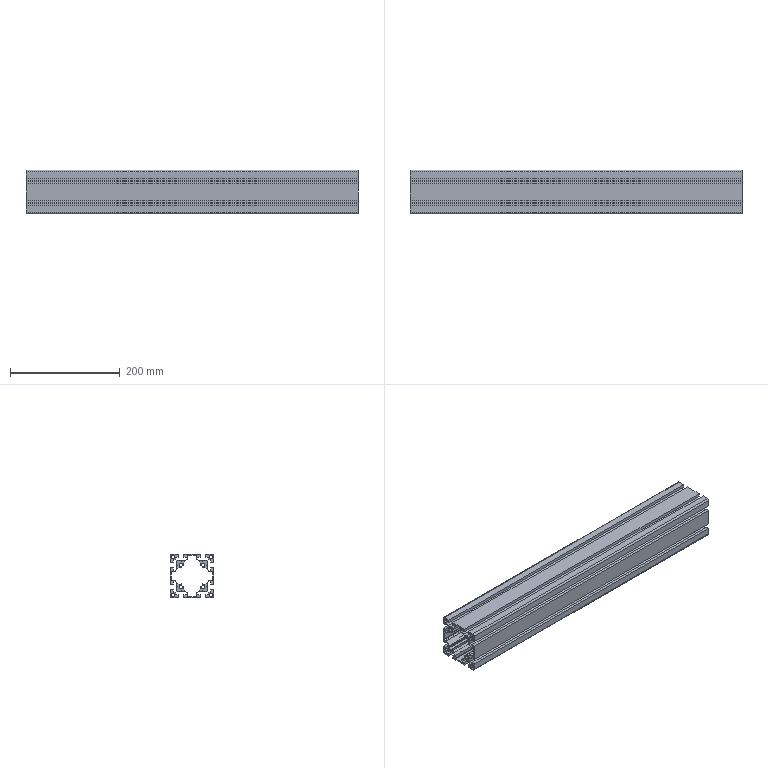Part | STEP file | PN_0062_Default<machined> | 1 solid | 204 faces | box 606 x 80 x 80 mm | volume 921943 mm3 | plane 154 | cylinder 50 | commonest cylinder face diameters 2 x24 6.8 x12 10.8 x10 6 x4